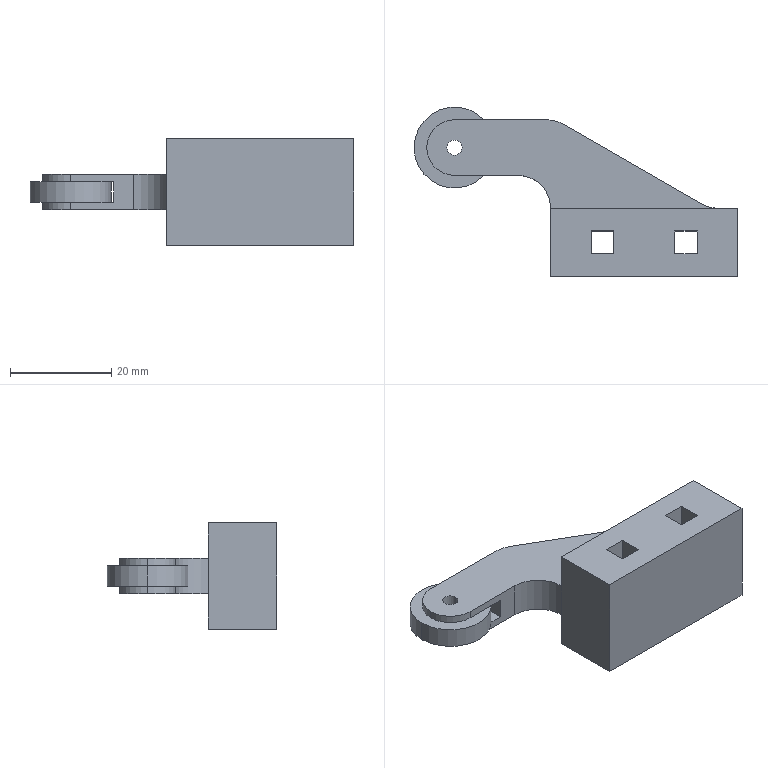Part | SolidWorks | features BaseBody 1 | 1 solid | 48 faces | box 64 x 33.5 x 21 mm | volume 12733 mm3 | plane 37 | cylinder 11 | commonest cylinder face diameters 11 x4 13 x3 3 x2 16 x2
STEP:
#1=CARTESIAN_POINT('',(-48.,25.5,2.));
#2=VERTEX_POINT('',#1);
#3=CARTESIAN_POINT('',(-50.191,31.,2.));
#4=VERTEX_POINT('',#3);
#5=CARTESIAN_POINT('',(-56.,25.5,2.));
#6=DIRECTION('',(0.,0.,1.));
#7=DIRECTION('',(1.,0.,0.));
#8=AXIS2_PLACEMENT_3D('',#5,#6,#7);
#9=CIRCLE('',#8,8.);
#10=EDGE_CURVE('',#2,#4,#9,.T.);
#11=ORIENTED_EDGE('',*,*,#10,.F.);
#12=CARTESIAN_POINT('',(-48.,25.5,-2.));
#13=VERTEX_POINT('',#12);
#14=CARTESIAN_POINT('',(-48.,25.5,2.));
#15=DIRECTION('',(0.,0.,-1.));
#16=VECTOR('',#15,1000.);
#17=LINE('',#14,#16);
#18=EDGE_CURVE('',#2,#13,#17,.T.);
#19=ORIENTED_EDGE('',*,*,#18,.T.);
#20=CARTESIAN_POINT('',(-50.191,31.,-2.));
#21=VERTEX_POINT('',#20);
#22=CARTESIAN_POINT('',(-56.,25.5,-2.));
#23=DIRECTION('',(0.,0.,1.));
#24=DIRECTION('',(-1.,0.,0.));
#25=AXIS2_PLACEMENT_3D('',#22,#23,#24);
#26=CIRCLE('',#25,8.);
#27=EDGE_CURVE('',#13,#21,#26,.T.);
#28=ORIENTED_EDGE('',*,*,#27,.T.);
#29=CARTESIAN_POINT('',(-64.,25.5,-2.));
#30=VERTEX_POINT('',#29);
#31=CARTESIAN_POINT('',(-56.,25.5,-2.));
#32=DIRECTION('',(0.,0.,1.));
#33=DIRECTION('',(1.,0.,0.));
#34=AXIS2_PLACEMENT_3D('',#31,#32,#33);
#35=CIRCLE('',#34,8.);
#36=EDGE_CURVE('',#21,#30,#35,.T.);
#37=ORIENTED_EDGE('',*,*,#36,.T.);
#38=CARTESIAN_POINT('',(-64.,25.5,2.));
#39=VERTEX_POINT('',#38);
#40=CARTESIAN_POINT('',(-64.,25.5,2.));
#41=DIRECTION('',(0.,0.,-1.));
#42=VECTOR('',#41,1000.);
#43=LINE('',#40,#42);
#44=EDGE_CURVE('',#39,#30,#43,.T.);
#45=ORIENTED_EDGE('',*,*,#44,.F.);
#46=CARTESIAN_POINT('',(-56.,25.5,2.));
#47=DIRECTION('',(0.,0.,1.));
#48=DIRECTION('',(1.,0.,0.));
#49=AXIS2_PLACEMENT_3D('',#46,#47,#48);
#50=CIRCLE('',#49,8.);
#51=EDGE_CURVE('',#4,#39,#50,.T.);
#52=ORIENTED_EDGE('',*,*,#51,.F.);
#53=EDGE_LOOP('',(#11,#19,#28,#37,#45,#52));
#54=FACE_OUTER_BOUND('',#53,.T.);
#55=CARTESIAN_POINT('',(-56.,25.5,2.));
#56=DIRECTION('',(0.,0.,-1.));
#57=DIRECTION('',(-1.,0.,0.));
#58=AXIS2_PLACEMENT_3D('',#55,#56,#57);
#59=CYLINDRICAL_SURFACE('',#58,8.);
#60=ADVANCED_FACE('',(#54),#59,.T.);
#61=CARTESIAN_POINT('',(-57.5,25.5,3.5));
#62=VERTEX_POINT('',#61);
#63=CARTESIAN_POINT('',(-54.5,25.5,3.5));
#64=VERTEX_POINT('',#63);
#65=CARTESIAN_POINT('',(-56.,25.5,3.5));
#66=DIRECTION('',(0.,0.,1.));
#67=DIRECTION('',(1.,0.,0.));
#68=AXIS2_PLACEMENT_3D('',#65,#66,#67);
#69=CIRCLE('',#68,1.5);
#70=EDGE_CURVE('',#62,#64,#69,.T.);
#71=ORIENTED_EDGE('',*,*,#70,.T.);
#72=CARTESIAN_POINT('',(-54.5,25.5,-3.5));
#73=VERTEX_POINT('',#72);
#74=CARTESIAN_POINT('',(-54.5,25.5,3.5));
#75=DIRECTION('',(0.,0.,-1.));
#76=VECTOR('',#75,1000.);
#77=LINE('',#74,#76);
#78=EDGE_CURVE('',#64,#73,#77,.T.);
#79=ORIENTED_EDGE('',*,*,#78,.T.);
#80=CARTESIAN_POINT('',(-57.5,25.5,-3.5));
#81=VERTEX_POINT('',#80);
#82=CARTESIAN_POINT('',(-56.,25.5,-3.5));
#83=DIRECTION('',(0.,0.,1.));
#84=DIRECTION('',(1.,0.,0.));
#85=AXIS2_PLACEMENT_3D('',#82,#83,#84);
#86=CIRCLE('',#85,1.5);
#87=EDGE_CURVE('',#81,#73,#86,.T.);
#88=ORIENTED_EDGE('',*,*,#87,.F.);
#89=CARTESIAN_POINT('',(-57.5,25.5,3.5));
#90=DIRECTION('',(0.,0.,-1.));
#91=VECTOR('',#90,1000.);
#92=LINE('',#89,#91);
#93=EDGE_CURVE('',#62,#81,#92,.T.);
#94=ORIENTED_EDGE('',*,*,#93,.F.);
#95=EDGE_LOOP('',(#71,#79,#88,#94));
#96=FACE_OUTER_BOUND('',#95,.T.);
#97=CARTESIAN_POINT('',(-56.,25.5,3.5));
#98=DIRECTION('',(0.,0.,-1.));
#99=DIRECTION('',(-1.,0.,0.));
#100=AXIS2_PLACEMENT_3D('',#97,#98,#99);
#101=CYLINDRICAL_SURFACE('',#100,1.5);
#102=ADVANCED_FACE('',(#96),#101,.F.);
#103=CARTESIAN_POINT('',(-56.,20.,-2.));
#104=VERTEX_POINT('',#103);
#105=CARTESIAN_POINT('',(-61.5,25.5,-2.));
#106=VERTEX_POINT('',#105);
#107=CARTESIAN_POINT('',(-56.,25.5,-2.));
#108=DIRECTION('',(0.,0.,-1.));
#109=DIRECTION('',(-1.,0.,0.));
#110=AXIS2_PLACEMENT_3D('',#107,#108,#109);
#111=CIRCLE('',#110,5.5);
#112=EDGE_CURVE('',#104,#106,#111,.T.);
#113=ORIENTED_EDGE('',*,*,#112,.T.);
#114=CARTESIAN_POINT('',(-61.5,25.5,-3.5));
#115=VERTEX_POINT('',#114);
#116=CARTESIAN_POINT('',(-61.5,25.5,3.5));
#117=DIRECTION('',(0.,0.,-1.));
#118=VECTOR('',#117,1000.);
#119=LINE('',#116,#118);
#120=EDGE_CURVE('',#106,#115,#119,.T.);
#121=ORIENTED_EDGE('',*,*,#120,.T.);
#122=CARTESIAN_POINT('',(-56.,20.,-3.5));
#123=VERTEX_POINT('',#122);
#124=CARTESIAN_POINT('',(-56.,25.5,-3.5));
#125=DIRECTION('',(0.,0.,1.));
#126=DIRECTION('',(1.,0.,0.));
#127=AXIS2_PLACEMENT_3D('',#124,#125,#126);
#128=CIRCLE('',#127,5.5);
#129=EDGE_CURVE('',#115,#123,#128,.T.);
#130=ORIENTED_EDGE('',*,*,#129,.T.);
#131=CARTESIAN_POINT('',(-56.,20.,3.5));
#132=DIRECTION('',(0.,0.,-1.));
#133=VECTOR('',#132,1000.);
#134=LINE('',#131,#133);
#135=EDGE_CURVE('',#104,#123,#134,.T.);
#136=ORIENTED_EDGE('',*,*,#135,.F.);
#137=EDGE_LOOP('',(#113,#121,#130,#136));
#138=FACE_OUTER_BOUND('',#137,.T.);
#139=CARTESIAN_POINT('',(-56.,25.5,3.5));
#140=DIRECTION('',(0.,0.,-1.));
#141=DIRECTION('',(-1.,0.,0.));
#142=AXIS2_PLACEMENT_3D('',#139,#140,#141);
#143=CYLINDRICAL_SURFACE('',#142,5.5);
#144=ADVANCED_FACE('',(#138),#143,.T.);
#145=CARTESIAN_POINT('',(-61.5,25.5,3.5));
#146=VERTEX_POINT('',#145);
#147=CARTESIAN_POINT('',(-56.,20.,3.5));
#148=VERTEX_POINT('',#147);
#149=CARTESIAN_POINT('',(-56.,25.5,3.5));
#150=DIRECTION('',(0.,0.,1.));
#151=DIRECTION('',(1.,0.,0.));
#152=AXIS2_PLACEMENT_3D('',#149,#150,#151);
#153=CIRCLE('',#152,5.5);
#154=EDGE_CURVE('',#146,#148,#153,.T.);
#155=ORIENTED_EDGE('',*,*,#154,.F.);
#156=CARTESIAN_POINT('',(-61.5,25.5,2.));
#157=VERTEX_POINT('',#156);
#158=CARTESIAN_POINT('',(-61.5,25.5,3.5));
#159=DIRECTION('',(0.,0.,-1.));
#160=VECTOR('',#159,1000.);
#161=LINE('',#158,#160);
#162=EDGE_CURVE('',#146,#157,#161,.T.);
#163=ORIENTED_EDGE('',*,*,#162,.T.);
#164=CARTESIAN_POINT('',(-56.,20.,2.));
#165=VERTEX_POINT('',#164);
#166=CARTESIAN_POINT('',(-56.,25.5,2.));
#167=DIRECTION('',(0.,0.,1.));
#168=DIRECTION('',(1.,0.,0.));
#169=AXIS2_PLACEMENT_3D('',#166,#167,#168);
#170=CIRCLE('',#169,5.5);
#171=EDGE_CURVE('',#157,#165,#170,.T.);
#172=ORIENTED_EDGE('',*,*,#171,.T.);
#173=CARTESIAN_POINT('',(-56.,20.,3.5));
#174=DIRECTION('',(0.,0.,-1.));
#175=VECTOR('',#174,1000.);
#176=LINE('',#173,#175);
#177=EDGE_CURVE('',#148,#165,#176,.T.);
#178=ORIENTED_EDGE('',*,*,#177,.F.);
#179=EDGE_LOOP('',(#155,#163,#172,#178));
#180=FACE_OUTER_BOUND('',#179,.T.);
#181=CARTESIAN_POINT('',(-56.,25.5,3.5));
#182=DIRECTION('',(0.,0.,-1.));
#183=DIRECTION('',(-1.,0.,0.));
#184=AXIS2_PLACEMENT_3D('',#181,#182,#183);
#185=CYLINDRICAL_SURFACE('',#184,5.5);
#186=ADVANCED_FACE('',(#180),#185,.T.);
#187=CARTESIAN_POINT('',(-8.,9.,-1.5));
#188=VERTEX_POINT('',#187);
#189=CARTESIAN_POINT('',(-8.,4.5,-1.5));
#190=VERTEX_POINT('',#189);
#191=CARTESIAN_POINT('',(-8.,4.5,-1.5));
#192=DIRECTION('',(0.,-1.,0.));
#193=VECTOR('',#192,1000.);
#194=LINE('',#191,#193);
#195=EDGE_CURVE('',#188,#190,#194,.T.);
#196=ORIENTED_EDGE('',*,*,#195,.F.);
#197=CARTESIAN_POINT('',(-8.,9.,-10.5));
#198=VERTEX_POINT('',#197);
#199=CARTESIAN_POINT('',(-8.,9.,3.5));
#200=DIRECTION('',(0.,0.,-1.));
#201=VECTOR('',#200,1000.);
#202=LINE('',#199,#201);
#203=EDGE_CURVE('',#188,#198,#202,.T.);
#204=ORIENTED_EDGE('',*,*,#203,.T.);
#205=CARTESIAN_POINT('',(-8.,4.5,-10.5));
#206=VERTEX_POINT('',#205);
#207=CARTESIAN_POINT('',(-8.,9.,-10.5));
#208=DIRECTION('',(0.,1.,0.));
#209=VECTOR('',#208,1000.);
#210=LINE('',#207,#209);
#211=EDGE_CURVE('',#206,#198,#210,.T.);
#212=ORIENTED_EDGE('',*,*,#211,.F.);
#213=CARTESIAN_POINT('',(-8.,4.5,3.5));
#214=DIRECTION('',(0.,0.,-1.));
#215=VECTOR('',#214,1000.);
#216=LINE('',#213,#215);
#217=EDGE_CURVE('',#190,#206,#216,.T.);
#218=ORIENTED_EDGE('',*,*,#217,.F.);
#219=EDGE_LOOP('',(#196,#204,#212,#218));
#220=FACE_OUTER_BOUND('',#219,.T.);
#221=CARTESIAN_POINT('',(-8.,4.5,3.5));
#222=DIRECTION('',(-1.,0.,0.));
#223=DIRECTION('',(0.,0.,1.));
#224=AXIS2_PLACEMENT_3D('',#221,#222,#223);
#225=PLANE('',#224);
#226=ADVANCED_FACE('',(#220),#225,.T.);
#227=CARTESIAN_POINT('',(-12.5,9.,-1.5));
#228=VERTEX_POINT('',#227);
#229=CARTESIAN_POINT('',(-12.5,9.,-1.5));
#230=DIRECTION('',(1.,0.,0.));
#231=VECTOR('',#230,1000.);
#232=LINE('',#229,#231);
#233=EDGE_CURVE('',#228,#188,#232,.T.);
#234=ORIENTED_EDGE('',*,*,#233,.F.);
#235=CARTESIAN_POINT('',(-12.5,9.,-10.5));
#236=VERTEX_POINT('',#235);
#237=CARTESIAN_POINT('',(-12.5,9.,3.5));
#238=DIRECTION('',(0.,0.,-1.));
#239=VECTOR('',#238,1000.);
#240=LINE('',#237,#239);
#241=EDGE_CURVE('',#228,#236,#240,.T.);
#242=ORIENTED_EDGE('',*,*,#241,.T.);
#243=CARTESIAN_POINT('',(-12.5,9.,-10.5));
#244=DIRECTION('',(-1.,0.,0.));
#245=VECTOR('',#244,1000.);
#246=LINE('',#243,#245);
#247=EDGE_CURVE('',#198,#236,#246,.T.);
#248=ORIENTED_EDGE('',*,*,#247,.F.);
#249=ORIENTED_EDGE('',*,*,#203,.F.);
#250=EDGE_LOOP('',(#234,#242,#248,#249));
#251=FACE_OUTER_BOUND('',#250,.T.);
#252=CARTESIAN_POINT('',(-12.5,9.,3.5));
#253=DIRECTION('',(0.,-1.,0.));
#254=DIRECTION('',(0.,0.,-1.));
#255=AXIS2_PLACEMENT_3D('',#252,#253,#254);
#256=PLANE('',#255);
#257=ADVANCED_FACE('',(#251),#256,.T.);
#258=CARTESIAN_POINT('',(-12.5,4.5,-1.5));
#259=VERTEX_POINT('',#258);
#260=CARTESIAN_POINT('',(-12.5,4.5,-1.5));
#261=DIRECTION('',(0.,1.,0.));
#262=VECTOR('',#261,1000.);
#263=LINE('',#260,#262);
#264=EDGE_CURVE('',#259,#228,#263,.T.);
#265=ORIENTED_EDGE('',*,*,#264,.F.);
#266=CARTESIAN_POINT('',(-12.5,4.5,-10.5));
#267=VERTEX_POINT('',#266);
#268=CARTESIAN_POINT('',(-12.5,4.5,3.5));
#269=DIRECTION('',(0.,0.,-1.));
#270=VECTOR('',#269,1000.);
#271=LINE('',#268,#270);
#272=EDGE_CURVE('',#259,#267,#271,.T.);
#273=ORIENTED_EDGE('',*,*,#272,.T.);
#274=CARTESIAN_POINT('',(-12.5,9.,-10.5));
#275=DIRECTION('',(0.,-1.,0.));
#276=VECTOR('',#275,1000.);
#277=LINE('',#274,#276);
#278=EDGE_CURVE('',#236,#267,#277,.T.);
#279=ORIENTED_EDGE('',*,*,#278,.F.);
#280=ORIENTED_EDGE('',*,*,#241,.F.);
#281=EDGE_LOOP('',(#265,#273,#279,#280));
#282=FACE_OUTER_BOUND('',#281,.T.);
#283=CARTESIAN_POINT('',(-12.5,4.5,3.5));
#284=DIRECTION('',(1.,0.,0.));
#285=DIRECTION('',(0.,1.,0.));
#286=AXIS2_PLACEMENT_3D('',#283,#284,#285);
#287=PLANE('',#286);
#288=ADVANCED_FACE('',(#282),#287,.T.);
#289=CARTESIAN_POINT('',(-12.5,4.5,-1.5));
#290=DIRECTION('',(-1.,0.,0.));
#291=VECTOR('',#290,1000.);
#292=LINE('',#289,#291);
#293=EDGE_CURVE('',#190,#259,#292,.T.);
#294=ORIENTED_EDGE('',*,*,#293,.F.);
#295=ORIENTED_EDGE('',*,*,#217,.T.);
#296=CARTESIAN_POINT('',(-12.5,4.5,-10.5));
#297=DIRECTION('',(1.,0.,0.));
#298=VECTOR('',#297,1000.);
#299=LINE('',#296,#298);
#300=EDGE_CURVE('',#267,#206,#299,.T.);
#301=ORIENTED_EDGE('',*,*,#300,.F.);
#302=ORIENTED_EDGE('',*,*,#272,.F.);
#303=EDGE_LOOP('',(#294,#295,#301,#302));
#304=FACE_OUTER_BOUND('',#303,.T.);
#305=CARTESIAN_POINT('',(-12.5,4.5,3.5));
#306=DIRECTION('',(0.,1.,0.));
#307=DIRECTION('',(1.,0.,0.));
#308=AXIS2_PLACEMENT_3D('',#305,#306,#307);
#309=PLANE('',#308);
#310=ADVANCED_FACE('',(#304),#309,.T.);
#311=CARTESIAN_POINT('',(-24.5,9.,-1.5));
#312=VERTEX_POINT('',#311);
#313=CARTESIAN_POINT('',(-24.5,4.5,-1.5));
#314=VERTEX_POINT('',#313);
#315=CARTESIAN_POINT('',(-24.5,4.5,-1.5));
#316=DIRECTION('',(0.,-1.,0.));
#317=VECTOR('',#316,1000.);
#318=LINE('',#315,#317);
#319=EDGE_CURVE('',#312,#314,#318,.T.);
#320=ORIENTED_EDGE('',*,*,#319,.F.);
#321=CARTESIAN_POINT('',(-24.5,9.,-10.5));
#322=VERTEX_POINT('',#321);
#323=CARTESIAN_POINT('',(-24.5,9.,3.5));
#324=DIRECTION('',(0.,0.,-1.));
#325=VECTOR('',#324,1000.);
#326=LINE('',#323,#325);
#327=EDGE_CURVE('',#312,#322,#326,.T.);
#328=ORIENTED_EDGE('',*,*,#327,.T.);
#329=CARTESIAN_POINT('',(-24.5,4.5,-10.5));
#330=VERTEX_POINT('',#329);
#331=CARTESIAN_POINT('',(-24.5,9.,-10.5));
#332=DIRECTION('',(0.,1.,0.));
#333=VECTOR('',#332,1000.);
#334=LINE('',#331,#333);
#335=EDGE_CURVE('',#330,#322,#334,.T.);
#336=ORIENTED_EDGE('',*,*,#335,.F.);
#337=CARTESIAN_POINT('',(-24.5,4.5,3.5));
#338=DIRECTION('',(0.,0.,-1.));
#339=VECTOR('',#338,1000.);
#340=LINE('',#337,#339);
#341=EDGE_CURVE('',#314,#330,#340,.T.);
#342=ORIENTED_EDGE('',*,*,#341,.F.);
#343=EDGE_LOOP('',(#320,#328,#336,#342));
#344=FACE_OUTER_BOUND('',#343,.T.);
#345=CARTESIAN_POINT('',(-24.5,4.5,3.5));
#346=DIRECTION('',(-1.,0.,0.));
#347=DIRECTION('',(0.,1.,0.));
#348=AXIS2_PLACEMENT_3D('',#345,#346,#347);
#349=PLANE('',#348);
#350=ADVANCED_FACE('',(#344),#349,.T.);
#351=CARTESIAN_POINT('',(-29.,9.,-1.5));
#352=VERTEX_POINT('',#351);
#353=CARTESIAN_POINT('',(-29.,9.,-1.5));
#354=DIRECTION('',(1.,0.,0.));
#355=VECTOR('',#354,1000.);
#356=LINE('',#353,#355);
#357=EDGE_CURVE('',#352,#312,#356,.T.);
#358=ORIENTED_EDGE('',*,*,#357,.F.);
#359=CARTESIAN_POINT('',(-29.,9.,-10.5));
#360=VERTEX_POINT('',#359);
#361=CARTESIAN_POINT('',(-29.,9.,3.5));
#362=DIRECTION('',(0.,0.,-1.));
#363=VECTOR('',#362,1000.);
#364=LINE('',#361,#363);
#365=EDGE_CURVE('',#352,#360,#364,.T.);
#366=ORIENTED_EDGE('',*,*,#365,.T.);
#367=CARTESIAN_POINT('',(-29.,9.,-10.5));
#368=DIRECTION('',(-1.,0.,0.));
#369=VECTOR('',#368,1000.);
#370=LINE('',#367,#369);
#371=EDGE_CURVE('',#322,#360,#370,.T.);
#372=ORIENTED_EDGE('',*,*,#371,.F.);
#373=ORIENTED_EDGE('',*,*,#327,.F.);
#374=EDGE_LOOP('',(#358,#366,#372,#373));
#375=FACE_OUTER_BOUND('',#374,.T.);
#376=CARTESIAN_POINT('',(-29.,9.,3.5));
#377=DIRECTION('',(0.,-1.,0.));
#378=DIRECTION('',(0.,0.,-1.));
#379=AXIS2_PLACEMENT_3D('',#376,#377,#378);
#380=PLANE('',#379);
#381=ADVANCED_FACE('',(#375),#380,.T.);
#382=CARTESIAN_POINT('',(-29.,4.5,-1.5));
#383=VERTEX_POINT('',#382);
#384=CARTESIAN_POINT('',(-29.,4.5,-1.5));
#385=DIRECTION('',(0.,1.,0.));
#386=VECTOR('',#385,1000.);
#387=LINE('',#384,#386);
#388=EDGE_CURVE('',#383,#352,#387,.T.);
#389=ORIENTED_EDGE('',*,*,#388,.F.);
#390=CARTESIAN_POINT('',(-29.,4.5,-10.5));
#391=VERTEX_POINT('',#390);
#392=CARTESIAN_POINT('',(-29.,4.5,3.5));
#393=DIRECTION('',(0.,0.,-1.));
#394=VECTOR('',#393,1000.);
#395=LINE('',#392,#394);
#396=EDGE_CURVE('',#383,#391,#395,.T.);
#397=ORIENTED_EDGE('',*,*,#396,.T.);
#398=CARTESIAN_POINT('',(-29.,9.,-10.5));
#399=DIRECTION('',(0.,-1.,0.));
#400=VECTOR('',#399,1000.);
#401=LINE('',#398,#400);
#402=EDGE_CURVE('',#360,#391,#401,.T.);
#403=ORIENTED_EDGE('',*,*,#402,.F.);
#404=ORIENTED_EDGE('',*,*,#365,.F.);
#405=EDGE_LOOP('',(#389,#397,#403,#404));
#406=FACE_OUTER_BOUND('',#405,.T.);
#407=CARTESIAN_POINT('',(-29.,4.5,3.5));
#408=DIRECTION('',(1.,0.,0.));
#409=DIRECTION('',(0.,1.,0.));
#410=AXIS2_PLACEMENT_3D('',#407,#408,#409);
#411=PLANE('',#410);
#412=ADVANCED_FACE('',(#406),#411,.T.);
#413=CARTESIAN_POINT('',(-29.,4.5,-1.5));
#414=DIRECTION('',(-1.,0.,0.));
#415=VECTOR('',#414,1000.);
#416=LINE('',#413,#415);
#417=EDGE_CURVE('',#314,#383,#416,.T.);
#418=ORIENTED_EDGE('',*,*,#417,.F.);
#419=ORIENTED_EDGE('',*,*,#341,.T.);
#420=CARTESIAN_POINT('',(-29.,4.5,-10.5));
#421=DIRECTION('',(1.,0.,0.));
#422=VECTOR('',#421,1000.);
#423=LINE('',#420,#422);
#424=EDGE_CURVE('',#391,#330,#423,.T.);
#425=ORIENTED_EDGE('',*,*,#424,.F.);
#426=ORIENTED_EDGE('',*,*,#396,.F.);
#427=EDGE_LOOP('',(#418,#419,#425,#426));
#428=FACE_OUTER_BOUND('',#427,.T.);
#429=CARTESIAN_POINT('',(-29.,4.5,3.5));
#430=DIRECTION('',(0.,1.,0.));
#431=DIRECTION('',(1.,0.,0.));
#432=AXIS2_PLACEMENT_3D('',#429,#430,#431);
#433=PLANE('',#432);
#434=ADVANCED_FACE('',(#428),#433,.T.);
#435=CARTESIAN_POINT('',(-50.191,20.,2.));
#436=VERTEX_POINT('',#435);
#437=CARTESIAN_POINT('',(-56.,25.5,2.));
#438=DIRECTION('',(0.,0.,1.));
#439=DIRECTION('',(1.,0.,0.));
#440=AXIS2_PLACEMENT_3D('',#437,#438,#439);
#441=CIRCLE('',#440,8.);
#442=EDGE_CURVE('',#436,#2,#441,.T.);
#443=ORIENTED_EDGE('',*,*,#442,.T.);
#444=ORIENTED_EDGE('',*,*,#10,.T.);
#445=CARTESIAN_POINT('',(-47.5,31.,2.));
#446=VERTEX_POINT('',#445);
#447=CARTESIAN_POINT('',(-56.,31.,2.));
#448=DIRECTION('',(-1.,0.,0.));
#449=VECTOR('',#448,1000.);
#450=LINE('',#447,#449);
#451=EDGE_CURVE('',#446,#4,#450,.T.);
#452=ORIENTED_EDGE('',*,*,#451,.F.);
#453=CARTESIAN_POINT('',(-47.5,20.,2.));
#454=VERTEX_POINT('',#453);
#455=CARTESIAN_POINT('',(-47.5,0.,2.));
#456=DIRECTION('',(0.,1.,0.));
#457=VECTOR('',#456,1000.);
#458=LINE('',#455,#457);
#459=EDGE_CURVE('',#454,#446,#458,.T.);
#460=ORIENTED_EDGE('',*,*,#459,.F.);
#461=CARTESIAN_POINT('',(-43.5,20.,2.));
#462=DIRECTION('',(1.,0.,0.));
#463=VECTOR('',#462,1000.);
#464=LINE('',#461,#463);
#465=EDGE_CURVE('',#436,#454,#464,.T.);
#466=ORIENTED_EDGE('',*,*,#465,.F.);
#467=EDGE_LOOP('',(#443,#444,#452,#460,#466));
#468=FACE_OUTER_BOUND('',#467,.T.);
#469=CARTESIAN_POINT('',(-67.5,0.,2.));
#470=DIRECTION('',(0.,0.,1.));
#471=DIRECTION('',(1.,0.,0.));
#472=AXIS2_PLACEMENT_3D('',#469,#470,#471);
#473=PLANE('',#472);
#474=ADVANCED_FACE('',(#468),#473,.F.);
#475=CARTESIAN_POINT('',(-50.191,20.,-2.));
#476=VERTEX_POINT('',#475);
#477=CARTESIAN_POINT('',(-56.,25.5,-2.));
#478=DIRECTION('',(0.,0.,1.));
#479=DIRECTION('',(-1.,0.,0.));
#480=AXIS2_PLACEMENT_3D('',#477,#478,#479);
#481=CIRCLE('',#480,8.);
#482=EDGE_CURVE('',#476,#13,#481,.T.);
#483=ORIENTED_EDGE('',*,*,#482,.F.);
#484=CARTESIAN_POINT('',(-47.5,20.,-2.));
#485=VERTEX_POINT('',#484);
#486=CARTESIAN_POINT('',(-43.5,20.,-2.));
#487=DIRECTION('',(-1.,0.,0.));
#488=VECTOR('',#487,1000.);
#489=LINE('',#486,#488);
#490=EDGE_CURVE('',#485,#476,#489,.T.);
#491=ORIENTED_EDGE('',*,*,#490,.F.);
#492=CARTESIAN_POINT('',(-47.5,31.,-2.));
#493=VERTEX_POINT('',#492);
#494=CARTESIAN_POINT('',(-47.5,0.,-2.));
#495=DIRECTION('',(0.,1.,0.));
#496=VECTOR('',#495,1000.);
#497=LINE('',#494,#496);
#498=EDGE_CURVE('',#485,#493,#497,.T.);
#499=ORIENTED_EDGE('',*,*,#498,.T.);
#500=CARTESIAN_POINT('',(-56.,31.,-2.));
#501=DIRECTION('',(1.,0.,0.));
#502=VECTOR('',#501,1000.);
#503=LINE('',#500,#502);
#504=EDGE_CURVE('',#21,#493,#503,.T.);
#505=ORIENTED_EDGE('',*,*,#504,.F.);
#506=ORIENTED_EDGE('',*,*,#27,.F.);
#507=EDGE_LOOP('',(#483,#491,#499,#505,#506));
#508=FACE_OUTER_BOUND('',#507,.T.);
#509=CARTESIAN_POINT('',(-67.5,0.,-2.));
#510=DIRECTION('',(0.,0.,-1.));
#511=DIRECTION('',(0.,-1.,0.));
#512=AXIS2_PLACEMENT_3D('',#509,#510,#511);
#513=PLANE('',#512);
#514=ADVANCED_FACE('',(#508),#513,.F.);
#515=ORIENTED_EDGE('',*,*,#162,.F.);
#516=CARTESIAN_POINT('',(-56.,31.,3.5));
#517=VERTEX_POINT('',#516);
#518=CARTESIAN_POINT('',(-56.,25.5,3.5));
#519=DIRECTION('',(0.,0.,1.));
#520=DIRECTION('',(1.,0.,0.));
#521=AXIS2_PLACEMENT_3D('',#518,#519,#520);
#522=CIRCLE('',#521,5.5);
#523=EDGE_CURVE('',#517,#146,#522,.T.);
#524=ORIENTED_EDGE('',*,*,#523,.F.);
#525=CARTESIAN_POINT('',(-56.,31.,2.));
#526=VERTEX_POINT('',#525);
#527=CARTESIAN_POINT('',(-56.,31.,3.5));
#528=DIRECTION('',(0.,0.,-1.));
#529=VECTOR('',#528,1000.);
#530=LINE('',#527,#529);
#531=EDGE_CURVE('',#517,#526,#530,.T.);
#532=ORIENTED_EDGE('',*,*,#531,.T.);
#533=CARTESIAN_POINT('',(-56.,25.5,2.));
#534=DIRECTION('',(0.,0.,1.));
#535=DIRECTION('',(1.,0.,0.));
#536=AXIS2_PLACEMENT_3D('',#533,#534,#535);
#537=CIRCLE('',#536,5.5);
#538=EDGE_CURVE('',#526,#157,#537,.T.);
#539=ORIENTED_EDGE('',*,*,#538,.T.);
#540=EDGE_LOOP('',(#515,#524,#532,#539));
#541=FACE_OUTER_BOUND('',#540,.T.);
#542=CARTESIAN_POINT('',(-56.,25.5,3.5));
#543=DIRECTION('',(0.,0.,-1.));
#544=DIRECTION('',(-1.,0.,0.));
#545=AXIS2_PLACEMENT_3D('',#542,#543,#544);
#546=CYLINDRICAL_SURFACE('',#545,5.5);
#547=ADVANCED_FACE('',(#541),#546,.T.);
#548=ORIENTED_EDGE('',*,*,#70,.F.);
#549=CARTESIAN_POINT('',(-56.,25.5,3.5));
#550=DIRECTION('',(0.,0.,1.));
#551=DIRECTION('',(1.,0.,0.));
#552=AXIS2_PLACEMENT_3D('',#549,#550,#551);
#553=CIRCLE('',#552,1.5);
#554=EDGE_CURVE('',#64,#62,#553,.T.);
#555=ORIENTED_EDGE('',*,*,#554,.F.);
#556=EDGE_LOOP('',(#548,#555));
#557=FACE_BOUND('',#556,.T.);
#558=CARTESIAN_POINT('',(-4.,13.5,3.5));
#559=VERTEX_POINT('',#558);
#560=CARTESIAN_POINT('',(-37.,13.5,3.5));
#561=VERTEX_POINT('',#560);
#562=CARTESIAN_POINT('',(0.,13.5,3.5));
#563=DIRECTION('',(-1.,0.,0.));
#564=VECTOR('',#563,1000.);
#565=LINE('',#562,#564);
#566=EDGE_CURVE('',#559,#561,#565,.T.);
#567=ORIENTED_EDGE('',*,*,#566,.F.);
#568=CARTESIAN_POINT('',(-7.25,14.371,3.5));
#569=VERTEX_POINT('',#568);
#570=CARTESIAN_POINT('',(-4.,20.,3.5));
#571=DIRECTION('',(0.,0.,-1.));
#572=DIRECTION('',(-1.,0.,0.));
#573=AXIS2_PLACEMENT_3D('',#570,#571,#572);
#574=CIRCLE('',#573,6.5);
#575=EDGE_CURVE('',#559,#569,#574,.T.);
#576=ORIENTED_EDGE('',*,*,#575,.T.);
#577=CARTESIAN_POINT('',(-34.544,30.129,3.5));
#578=VERTEX_POINT('',#577);
#579=CARTESIAN_POINT('',(-34.544,30.129,3.5));
#580=DIRECTION('',(-0.866,0.5,0.));
#581=VECTOR('',#580,1000.);
#582=LINE('',#579,#581);
#583=EDGE_CURVE('',#569,#578,#582,.T.);
#584=ORIENTED_EDGE('',*,*,#583,.T.);
#585=CARTESIAN_POINT('',(-37.794,31.,3.5));
#586=VERTEX_POINT('',#585);
#587=CARTESIAN_POINT('',(-37.794,24.5,3.5));
#588=DIRECTION('',(0.,0.,1.));
#589=DIRECTION('',(1.,0.,0.));
#590=AXIS2_PLACEMENT_3D('',#587,#588,#589);
#591=CIRCLE('',#590,6.5);
#592=EDGE_CURVE('',#578,#586,#591,.T.);
#593=ORIENTED_EDGE('',*,*,#592,.T.);
#594=CARTESIAN_POINT('',(-56.,31.,3.5));
#595=DIRECTION('',(-1.,0.,0.));
#596=VECTOR('',#595,1000.);
#597=LINE('',#594,#596);
#598=EDGE_CURVE('',#586,#517,#597,.T.);
#599=ORIENTED_EDGE('',*,*,#598,.T.);
#600=ORIENTED_EDGE('',*,*,#523,.T.);
#601=ORIENTED_EDGE('',*,*,#154,.T.);
#602=CARTESIAN_POINT('',(-43.5,20.,3.5));
#603=VERTEX_POINT('',#602);
#604=CARTESIAN_POINT('',(-43.5,20.,3.5));
#605=DIRECTION('',(1.,0.,0.));
#606=VECTOR('',#605,1000.);
#607=LINE('',#604,#606);
#608=EDGE_CURVE('',#148,#603,#607,.T.);
#609=ORIENTED_EDGE('',*,*,#608,.T.);
#610=CARTESIAN_POINT('',(-43.5,13.5,3.5));
#611=DIRECTION('',(0.,0.,-1.));
#612=DIRECTION('',(1.,0.,0.));
#613=AXIS2_PLACEMENT_3D('',#610,#611,#612);
#614=CIRCLE('',#613,6.5);
#615=EDGE_CURVE('',#603,#561,#614,.T.);
#616=ORIENTED_EDGE('',*,*,#615,.T.);
#617=EDGE_LOOP('',(#567,#576,#584,#593,#599,#600,#601,#609,#616));
#618=FACE_OUTER_BOUND('',#617,.T.);
#619=CARTESIAN_POINT('',(-43.5,13.5,3.5));
#620=DIRECTION('',(0.,0.,1.));
#621=DIRECTION('',(1.,0.,0.));
#622=AXIS2_PLACEMENT_3D('',#619,#620,#621);
#623=PLANE('',#622);
#624=ADVANCED_FACE('',(#557,#618),#623,.T.);
#625=ORIENTED_EDGE('',*,*,#87,.T.);
#626=CARTESIAN_POINT('',(-56.,25.5,-3.5));
#627=DIRECTION('',(0.,0.,1.));
#628=DIRECTION('',(1.,0.,0.));
#629=AXIS2_PLACEMENT_3D('',#626,#627,#628);
#630=CIRCLE('',#629,1.5);
#631=EDGE_CURVE('',#73,#81,#630,.T.);
#632=ORIENTED_EDGE('',*,*,#631,.T.);
#633=EDGE_LOOP('',(#625,#632));
#634=FACE_BOUND('',#633,.T.);
#635=CARTESIAN_POINT('',(-4.,13.5,-3.5));
#636=VERTEX_POINT('',#635);
#637=CARTESIAN_POINT('',(-7.25,14.371,-3.5));
#638=VERTEX_POINT('',#637);
#639=CARTESIAN_POINT('',(-4.,20.,-3.5));
#640=DIRECTION('',(0.,0.,-1.));
#641=DIRECTION('',(-1.,0.,0.));
#642=AXIS2_PLACEMENT_3D('',#639,#640,#641);
#643=CIRCLE('',#642,6.5);
#644=EDGE_CURVE('',#636,#638,#643,.T.);
#645=ORIENTED_EDGE('',*,*,#644,.F.);
#646=CARTESIAN_POINT('',(-37.,13.5,-3.5));
#647=VERTEX_POINT('',#646);
#648=CARTESIAN_POINT('',(0.,13.5,-3.5));
#649=DIRECTION('',(-1.,0.,0.));
#650=VECTOR('',#649,1000.);
#651=LINE('',#648,#650);
#652=EDGE_CURVE('',#636,#647,#651,.T.);
#653=ORIENTED_EDGE('',*,*,#652,.T.);
#654=CARTESIAN_POINT('',(-43.5,20.,-3.5));
#655=VERTEX_POINT('',#654);
#656=CARTESIAN_POINT('',(-43.5,13.5,-3.5));
#657=DIRECTION('',(0.,0.,-1.));
#658=DIRECTION('',(1.,0.,0.));
#659=AXIS2_PLACEMENT_3D('',#656,#657,#658);
#660=CIRCLE('',#659,6.5);
#661=EDGE_CURVE('',#655,#647,#660,.T.);
#662=ORIENTED_EDGE('',*,*,#661,.F.);
#663=CARTESIAN_POINT('',(-43.5,20.,-3.5));
#664=DIRECTION('',(1.,0.,0.));
#665=VECTOR('',#664,1000.);
#666=LINE('',#663,#665);
#667=EDGE_CURVE('',#123,#655,#666,.T.);
#668=ORIENTED_EDGE('',*,*,#667,.F.);
#669=ORIENTED_EDGE('',*,*,#129,.F.);
#670=CARTESIAN_POINT('',(-56.,31.,-3.5));
#671=VERTEX_POINT('',#670);
#672=CARTESIAN_POINT('',(-56.,25.5,-3.5));
#673=DIRECTION('',(0.,0.,1.));
#674=DIRECTION('',(1.,0.,0.));
#675=AXIS2_PLACEMENT_3D('',#672,#673,#674);
#676=CIRCLE('',#675,5.5);
#677=EDGE_CURVE('',#671,#115,#676,.T.);
#678=ORIENTED_EDGE('',*,*,#677,.F.);
#679=CARTESIAN_POINT('',(-37.794,31.,-3.5));
#680=VERTEX_POINT('',#679);
#681=CARTESIAN_POINT('',(-56.,31.,-3.5));
#682=DIRECTION('',(-1.,0.,0.));
#683=VECTOR('',#682,1000.);
#684=LINE('',#681,#683);
#685=EDGE_CURVE('',#680,#671,#684,.T.);
#686=ORIENTED_EDGE('',*,*,#685,.F.);
#687=CARTESIAN_POINT('',(-34.544,30.129,-3.5));
#688=VERTEX_POINT('',#687);
#689=CARTESIAN_POINT('',(-37.794,24.5,-3.5));
#690=DIRECTION('',(0.,0.,1.));
#691=DIRECTION('',(1.,0.,0.));
#692=AXIS2_PLACEMENT_3D('',#689,#690,#691);
#693=CIRCLE('',#692,6.5);
#694=EDGE_CURVE('',#688,#680,#693,.T.);
#695=ORIENTED_EDGE('',*,*,#694,.F.);
#696=CARTESIAN_POINT('',(-34.544,30.129,-3.5));
#697=DIRECTION('',(-0.866,0.5,0.));
#698=VECTOR('',#697,1000.);
#699=LINE('',#696,#698);
#700=EDGE_CURVE('',#638,#688,#699,.T.);
#701=ORIENTED_EDGE('',*,*,#700,.F.);
#702=EDGE_LOOP('',(#645,#653,#662,#668,#669,#678,#686,#695,#701));
#703=FACE_OUTER_BOUND('',#702,.T.);
#704=CARTESIAN_POINT('',(-43.5,13.5,-3.5));
#705=DIRECTION('',(0.,0.,1.));
#706=DIRECTION('',(1.,0.,0.));
#707=AXIS2_PLACEMENT_3D('',#704,#705,#706);
#708=PLANE('',#707);
#709=ADVANCED_FACE('',(#634,#703),#708,.F.);
#710=CARTESIAN_POINT('',(0.,11.75,-1.5));
#711=VERTEX_POINT('',#710);
#712=CARTESIAN_POINT('',(0.,11.75,1.5));
#713=VERTEX_POINT('',#712);
#714=CARTESIAN_POINT('',(0.,11.75,1.5));
#715=DIRECTION('',(0.,0.,1.));
#716=VECTOR('',#715,1000.);
#717=LINE('',#714,#716);
#718=EDGE_CURVE('',#711,#713,#717,.T.);
#719=ORIENTED_EDGE('',*,*,#718,.F.);
#720=CARTESIAN_POINT('',(0.,1.75,-1.5));
#721=VERTEX_POINT('',#720);
#722=CARTESIAN_POINT('',(0.,1.75,-1.5));
#723=DIRECTION('',(0.,1.,0.));
#724=VECTOR('',#723,1000.);
#725=LINE('',#722,#724);
#726=EDGE_CURVE('',#721,#711,#725,.T.);
#727=ORIENTED_EDGE('',*,*,#726,.F.);
#728=CARTESIAN_POINT('',(0.,1.75,1.5));
#729=VERTEX_POINT('',#728);
#730=CARTESIAN_POINT('',(0.,1.75,1.5));
#731=DIRECTION('',(0.,0.,-1.));
#732=VECTOR('',#731,1000.);
#733=LINE('',#730,#732);
#734=EDGE_CURVE('',#729,#721,#733,.T.);
#735=ORIENTED_EDGE('',*,*,#734,.F.);
#736=CARTESIAN_POINT('',(0.,1.75,1.5));
#737=DIRECTION('',(0.,-1.,0.));
#738=VECTOR('',#737,1000.);
#739=LINE('',#736,#738);
#740=EDGE_CURVE('',#713,#729,#739,.T.);
#741=ORIENTED_EDGE('',*,*,#740,.F.);
#742=EDGE_LOOP('',(#719,#727,#735,#741));
#743=FACE_BOUND('',#742,.T.);
#744=CARTESIAN_POINT('',(0.,0.,10.5));
#745=VERTEX_POINT('',#744);
#746=CARTESIAN_POINT('',(0.,0.,-10.5));
#747=VERTEX_POINT('',#746);
#748=CARTESIAN_POINT('',(0.,0.,3.5));
#749=DIRECTION('',(0.,0.,-1.));
#750=VECTOR('',#749,1000.);
#751=LINE('',#748,#750);
#752=EDGE_CURVE('',#745,#747,#751,.T.);
#753=ORIENTED_EDGE('',*,*,#752,.T.);
#754=CARTESIAN_POINT('',(0.,13.5,-10.5));
#755=VERTEX_POINT('',#754);
#756=CARTESIAN_POINT('',(0.,13.5,-10.5));
#757=DIRECTION('',(0.,1.,0.));
#758=VECTOR('',#757,1000.);
#759=LINE('',#756,#758);
#760=EDGE_CURVE('',#747,#755,#759,.T.);
#761=ORIENTED_EDGE('',*,*,#760,.T.);
#762=CARTESIAN_POINT('',(0.,13.5,10.5));
#763=VERTEX_POINT('',#762);
#764=CARTESIAN_POINT('',(0.,13.5,3.5));
#765=DIRECTION('',(0.,0.,-1.));
#766=VECTOR('',#765,1000.);
#767=LINE('',#764,#766);
#768=EDGE_CURVE('',#763,#755,#767,.T.);
#769=ORIENTED_EDGE('',*,*,#768,.F.);
#770=CARTESIAN_POINT('',(0.,13.5,10.5));
#771=DIRECTION('',(0.,1.,0.));
#772=VECTOR('',#771,1000.);
#773=LINE('',#770,#772);
#774=EDGE_CURVE('',#745,#763,#773,.T.);
#775=ORIENTED_EDGE('',*,*,#774,.F.);
#776=EDGE_LOOP('',(#753,#761,#769,#775));
#777=FACE_OUTER_BOUND('',#776,.T.);
#778=CARTESIAN_POINT('',(0.,13.5,3.5));
#779=DIRECTION('',(-1.,0.,0.));
#780=DIRECTION('',(0.,1.,0.));
#781=AXIS2_PLACEMENT_3D('',#778,#779,#780);
#782=PLANE('',#781);
#783=ADVANCED_FACE('',(#743,#777),#782,.F.);
#784=ORIENTED_EDGE('',*,*,#768,.T.);
#785=CARTESIAN_POINT('',(-37.,13.5,-10.5));
#786=VERTEX_POINT('',#785);
#787=CARTESIAN_POINT('',(0.,13.5,-10.5));
#788=DIRECTION('',(-1.,0.,0.));
#789=VECTOR('',#788,1000.);
#790=LINE('',#787,#789);
#791=EDGE_CURVE('',#755,#786,#790,.T.);
#792=ORIENTED_EDGE('',*,*,#791,.T.);
#793=CARTESIAN_POINT('',(-37.,13.5,-10.5));
#794=DIRECTION('',(0.,0.,1.));
#795=VECTOR('',#794,1000.);
#796=LINE('',#793,#795);
#797=EDGE_CURVE('',#786,#647,#796,.T.);
#798=ORIENTED_EDGE('',*,*,#797,.T.);
#799=ORIENTED_EDGE('',*,*,#652,.F.);
#800=CARTESIAN_POINT('',(-4.,13.5,3.5));
#801=DIRECTION('',(0.,0.,-1.));
#802=VECTOR('',#801,1000.);
#803=LINE('',#800,#802);
#804=EDGE_CURVE('',#559,#636,#803,.T.);
#805=ORIENTED_EDGE('',*,*,#804,.F.);
#806=ORIENTED_EDGE('',*,*,#566,.T.);
#807=CARTESIAN_POINT('',(-37.,13.5,10.5));
#808=VERTEX_POINT('',#807);
#809=CARTESIAN_POINT('',(-37.,13.5,10.5));
#810=DIRECTION('',(0.,0.,-1.));
#811=VECTOR('',#810,1000.);
#812=LINE('',#809,#811);
#813=EDGE_CURVE('',#808,#561,#812,.T.);
#814=ORIENTED_EDGE('',*,*,#813,.F.);
#815=CARTESIAN_POINT('',(0.,13.5,10.5));
#816=DIRECTION('',(-1.,0.,0.));
#817=VECTOR('',#816,1000.);
#818=LINE('',#815,#817);
#819=EDGE_CURVE('',#763,#808,#818,.T.);
#820=ORIENTED_EDGE('',*,*,#819,.F.);
#821=EDGE_LOOP('',(#784,#792,#798,#799,#805,#806,#814,#820));
#822=FACE_OUTER_BOUND('',#821,.T.);
#823=CARTESIAN_POINT('',(-4.,13.5,3.5));
#824=DIRECTION('',(0.,-1.,0.));
#825=DIRECTION('',(0.,0.,-1.));
#826=AXIS2_PLACEMENT_3D('',#823,#824,#825);
#827=PLANE('',#826);
#828=ADVANCED_FACE('',(#822),#827,.F.);
#829=ORIENTED_EDGE('',*,*,#644,.T.);
#830=CARTESIAN_POINT('',(-7.25,14.371,3.5));
#831=DIRECTION('',(0.,0.,-1.));
#832=VECTOR('',#831,1000.);
#833=LINE('',#830,#832);
#834=EDGE_CURVE('',#569,#638,#833,.T.);
#835=ORIENTED_EDGE('',*,*,#834,.F.);
#836=ORIENTED_EDGE('',*,*,#575,.F.);
#837=ORIENTED_EDGE('',*,*,#804,.T.);
#838=EDGE_LOOP('',(#829,#835,#836,#837));
#839=FACE_OUTER_BOUND('',#838,.T.);
#840=CARTESIAN_POINT('',(-4.,20.,3.5));
#841=DIRECTION('',(0.,0.,-1.));
#842=DIRECTION('',(-1.,0.,0.));
#843=AXIS2_PLACEMENT_3D('',#840,#841,#842);
#844=CYLINDRICAL_SURFACE('',#843,6.5);
#845=ADVANCED_FACE('',(#839),#844,.F.);
#846=ORIENTED_EDGE('',*,*,#700,.T.);
#847=CARTESIAN_POINT('',(-34.544,30.129,3.5));
#848=DIRECTION('',(0.,0.,-1.));
#849=VECTOR('',#848,1000.);
#850=LINE('',#847,#849);
#851=EDGE_CURVE('',#578,#688,#850,.T.);
#852=ORIENTED_EDGE('',*,*,#851,.F.);
#853=ORIENTED_EDGE('',*,*,#583,.F.);
#854=ORIENTED_EDGE('',*,*,#834,.T.);
#855=EDGE_LOOP('',(#846,#852,#853,#854));
#856=FACE_OUTER_BOUND('',#855,.T.);
#857=CARTESIAN_POINT('',(-34.544,30.129,3.5));
#858=DIRECTION('',(-0.5,-0.866,0.));
#859=DIRECTION('',(-0.866,0.5,0.));
#860=AXIS2_PLACEMENT_3D('',#857,#858,#859);
#861=PLANE('',#860);
#862=ADVANCED_FACE('',(#856),#861,.F.);
#863=ORIENTED_EDGE('',*,*,#694,.T.);
#864=CARTESIAN_POINT('',(-37.794,31.,3.5));
#865=DIRECTION('',(0.,0.,-1.));
#866=VECTOR('',#865,1000.);
#867=LINE('',#864,#866);
#868=EDGE_CURVE('',#586,#680,#867,.T.);
#869=ORIENTED_EDGE('',*,*,#868,.F.);
#870=ORIENTED_EDGE('',*,*,#592,.F.);
#871=ORIENTED_EDGE('',*,*,#851,.T.);
#872=EDGE_LOOP('',(#863,#869,#870,#871));
#873=FACE_OUTER_BOUND('',#872,.T.);
#874=CARTESIAN_POINT('',(-37.794,24.5,3.5));
#875=DIRECTION('',(0.,0.,-1.));
#876=DIRECTION('',(-1.,0.,0.));
#877=AXIS2_PLACEMENT_3D('',#874,#875,#876);
#878=CYLINDRICAL_SURFACE('',#877,6.5);
#879=ADVANCED_FACE('',(#873),#878,.T.);
#880=CARTESIAN_POINT('',(-47.5,31.,3.5));
#881=DIRECTION('',(0.,0.,1.));
#882=VECTOR('',#881,1000.);
#883=LINE('',#880,#882);
#884=EDGE_CURVE('',#493,#446,#883,.T.);
#885=ORIENTED_EDGE('',*,*,#884,.T.);
#886=ORIENTED_EDGE('',*,*,#451,.T.);
#887=CARTESIAN_POINT('',(-56.,31.,2.));
#888=DIRECTION('',(-1.,0.,0.));
#889=VECTOR('',#888,1000.);
#890=LINE('',#887,#889);
#891=EDGE_CURVE('',#4,#526,#890,.T.);
#892=ORIENTED_EDGE('',*,*,#891,.T.);
#893=ORIENTED_EDGE('',*,*,#531,.F.);
#894=ORIENTED_EDGE('',*,*,#598,.F.);
#895=ORIENTED_EDGE('',*,*,#868,.T.);
#896=ORIENTED_EDGE('',*,*,#685,.T.);
#897=CARTESIAN_POINT('',(-56.,31.,-2.));
#898=VERTEX_POINT('',#897);
#899=CARTESIAN_POINT('',(-56.,31.,3.5));
#900=DIRECTION('',(0.,0.,-1.));
#901=VECTOR('',#900,1000.);
#902=LINE('',#899,#901);
#903=EDGE_CURVE('',#898,#671,#902,.T.);
#904=ORIENTED_EDGE('',*,*,#903,.F.);
#905=CARTESIAN_POINT('',(-56.,31.,-2.));
#906=DIRECTION('',(1.,0.,0.));
#907=VECTOR('',#906,1000.);
#908=LINE('',#905,#907);
#909=EDGE_CURVE('',#898,#21,#908,.T.);
#910=ORIENTED_EDGE('',*,*,#909,.T.);
#911=ORIENTED_EDGE('',*,*,#504,.T.);
#912=EDGE_LOOP('',(#885,#886,#892,#893,#894,#895,#896,#904,#910,#911));
#913=FACE_OUTER_BOUND('',#912,.T.);
#914=CARTESIAN_POINT('',(-56.,31.,3.5));
#915=DIRECTION('',(0.,-1.,0.));
#916=DIRECTION('',(0.,0.,-1.));
#917=AXIS2_PLACEMENT_3D('',#914,#915,#916);
#918=PLANE('',#917);
#919=ADVANCED_FACE('',(#913),#918,.F.);
#920=ORIENTED_EDGE('',*,*,#120,.F.);
#921=CARTESIAN_POINT('',(-56.,25.5,-2.));
#922=DIRECTION('',(0.,0.,-1.));
#923=DIRECTION('',(-1.,0.,0.));
#924=AXIS2_PLACEMENT_3D('',#921,#922,#923);
#925=CIRCLE('',#924,5.5);
#926=EDGE_CURVE('',#106,#898,#925,.T.);
#927=ORIENTED_EDGE('',*,*,#926,.T.);
#928=ORIENTED_EDGE('',*,*,#903,.T.);
#929=ORIENTED_EDGE('',*,*,#677,.T.);
#930=EDGE_LOOP('',(#920,#927,#928,#929));
#931=FACE_OUTER_BOUND('',#930,.T.);
#932=CARTESIAN_POINT('',(-56.,25.5,3.5));
#933=DIRECTION('',(0.,0.,-1.));
#934=DIRECTION('',(-1.,0.,0.));
#935=AXIS2_PLACEMENT_3D('',#932,#933,#934);
#936=CYLINDRICAL_SURFACE('',#935,5.5);
#937=ADVANCED_FACE('',(#931),#936,.T.);
#938=ORIENTED_EDGE('',*,*,#177,.T.);
#939=CARTESIAN_POINT('',(-43.5,20.,2.));
#940=DIRECTION('',(1.,0.,0.));
#941=VECTOR('',#940,1000.);
#942=LINE('',#939,#941);
#943=EDGE_CURVE('',#165,#436,#942,.T.);
#944=ORIENTED_EDGE('',*,*,#943,.T.);
#945=ORIENTED_EDGE('',*,*,#465,.T.);
#946=CARTESIAN_POINT('',(-47.5,20.,3.5));
#947=DIRECTION('',(0.,0.,-1.));
#948=VECTOR('',#947,1000.);
#949=LINE('',#946,#948);
#950=EDGE_CURVE('',#454,#485,#949,.T.);
#951=ORIENTED_EDGE('',*,*,#950,.T.);
#952=ORIENTED_EDGE('',*,*,#490,.T.);
#953=CARTESIAN_POINT('',(-43.5,20.,-2.));
#954=DIRECTION('',(-1.,0.,0.));
#955=VECTOR('',#954,1000.);
#956=LINE('',#953,#955);
#957=EDGE_CURVE('',#476,#104,#956,.T.);
#958=ORIENTED_EDGE('',*,*,#957,.T.);
#959=ORIENTED_EDGE('',*,*,#135,.T.);
#960=ORIENTED_EDGE('',*,*,#667,.T.);
#961=CARTESIAN_POINT('',(-43.5,20.,3.5));
#962=DIRECTION('',(0.,0.,-1.));
#963=VECTOR('',#962,1000.);
#964=LINE('',#961,#963);
#965=EDGE_CURVE('',#603,#655,#964,.T.);
#966=ORIENTED_EDGE('',*,*,#965,.F.);
#967=ORIENTED_EDGE('',*,*,#608,.F.);
#968=EDGE_LOOP('',(#938,#944,#945,#951,#952,#958,#959,#960,#966,#967));
#969=FACE_OUTER_BOUND('',#968,.T.);
#970=CARTESIAN_POINT('',(-43.5,20.,3.5));
#971=DIRECTION('',(0.,1.,0.));
#972=DIRECTION('',(1.,0.,0.));
#973=AXIS2_PLACEMENT_3D('',#970,#971,#972);
#974=PLANE('',#973);
#975=ADVANCED_FACE('',(#969),#974,.F.);
#976=ORIENTED_EDGE('',*,*,#661,.T.);
#977=CARTESIAN_POINT('',(-37.,13.5,3.5));
#978=DIRECTION('',(0.,0.,-1.));
#979=VECTOR('',#978,1000.);
#980=LINE('',#977,#979);
#981=EDGE_CURVE('',#561,#647,#980,.T.);
#982=ORIENTED_EDGE('',*,*,#981,.F.);
#983=ORIENTED_EDGE('',*,*,#615,.F.);
#984=ORIENTED_EDGE('',*,*,#965,.T.);
#985=EDGE_LOOP('',(#976,#982,#983,#984));
#986=FACE_OUTER_BOUND('',#985,.T.);
#987=CARTESIAN_POINT('',(-43.5,13.5,3.5));
#988=DIRECTION('',(0.,0.,-1.));
#989=DIRECTION('',(-1.,0.,0.));
#990=AXIS2_PLACEMENT_3D('',#987,#988,#989);
#991=CYLINDRICAL_SURFACE('',#990,6.5);
#992=ADVANCED_FACE('',(#986),#991,.F.);
#993=ORIENTED_EDGE('',*,*,#981,.T.);
#994=ORIENTED_EDGE('',*,*,#797,.F.);
#995=CARTESIAN_POINT('',(-37.,0.,-10.5));
#996=VERTEX_POINT('',#995);
#997=CARTESIAN_POINT('',(-37.,13.5,-10.5));
#998=DIRECTION('',(0.,-1.,0.));
#999=VECTOR('',#998,1000.);
#1000=LINE('',#997,#999);
#1001=EDGE_CURVE('',#786,#996,#1000,.T.);
#1002=ORIENTED_EDGE('',*,*,#1001,.T.);
#1003=CARTESIAN_POINT('',(-37.,0.,10.5));
#1004=VERTEX_POINT('',#1003);
#1005=CARTESIAN_POINT('',(-37.,0.,3.5));
#1006=DIRECTION('',(0.,0.,-1.));
#1007=VECTOR('',#1006,1000.);
#1008=LINE('',#1005,#1007);
#1009=EDGE_CURVE('',#1004,#996,#1008,.T.);
#1010=ORIENTED_EDGE('',*,*,#1009,.F.);
#1011=CARTESIAN_POINT('',(-37.,13.5,10.5));
#1012=DIRECTION('',(0.,-1.,0.));
#1013=VECTOR('',#1012,1000.);
#1014=LINE('',#1011,#1013);
#1015=EDGE_CURVE('',#808,#1004,#1014,.T.);
#1016=ORIENTED_EDGE('',*,*,#1015,.F.);
#1017=ORIENTED_EDGE('',*,*,#813,.T.);
#1018=EDGE_LOOP('',(#993,#994,#1002,#1010,#1016,#1017));
#1019=FACE_OUTER_BOUND('',#1018,.T.);
#1020=CARTESIAN_POINT('',(-37.,0.,3.5));
#1021=DIRECTION('',(1.,0.,0.));
#1022=DIRECTION('',(0.,1.,0.));
#1023=AXIS2_PLACEMENT_3D('',#1020,#1021,#1022);
#1024=PLANE('',#1023);
#1025=ADVANCED_FACE('',(#1019),#1024,.F.);
#1026=ORIENTED_EDGE('',*,*,#1009,.T.);
#1027=CARTESIAN_POINT('',(0.,0.,-10.5));
#1028=DIRECTION('',(1.,0.,0.));
#1029=VECTOR('',#1028,1000.);
#1030=LINE('',#1027,#1029);
#1031=EDGE_CURVE('',#996,#747,#1030,.T.);
#1032=ORIENTED_EDGE('',*,*,#1031,.T.);
#1033=ORIENTED_EDGE('',*,*,#752,.F.);
#1034=CARTESIAN_POINT('',(0.,0.,10.5));
#1035=DIRECTION('',(1.,0.,0.));
#1036=VECTOR('',#1035,1000.);
#1037=LINE('',#1034,#1036);
#1038=EDGE_CURVE('',#1004,#745,#1037,.T.);
#1039=ORIENTED_EDGE('',*,*,#1038,.F.);
#1040=EDGE_LOOP('',(#1026,#1032,#1033,#1039));
#1041=FACE_OUTER_BOUND('',#1040,.T.);
#1042=CARTESIAN_POINT('',(0.,0.,3.5));
#1043=DIRECTION('',(0.,1.,0.));
#1044=DIRECTION('',(1.,0.,0.));
#1045=AXIS2_PLACEMENT_3D('',#1042,#1043,#1044);
#1046=PLANE('',#1045);
#1047=ADVANCED_FACE('',(#1041),#1046,.F.);
#1048=ORIENTED_EDGE('',*,*,#78,.F.);
#1049=ORIENTED_EDGE('',*,*,#554,.T.);
#1050=ORIENTED_EDGE('',*,*,#93,.T.);
#1051=ORIENTED_EDGE('',*,*,#631,.F.);
#1052=EDGE_LOOP('',(#1048,#1049,#1050,#1051));
#1053=FACE_OUTER_BOUND('',#1052,.T.);
#1054=CARTESIAN_POINT('',(-56.,25.5,3.5));
#1055=DIRECTION('',(0.,0.,-1.));
#1056=DIRECTION('',(-1.,0.,0.));
#1057=AXIS2_PLACEMENT_3D('',#1054,#1055,#1056);
#1058=CYLINDRICAL_SURFACE('',#1057,1.5);
#1059=ADVANCED_FACE('',(#1053),#1058,.F.);
#1060=CARTESIAN_POINT('',(-8.,4.5,1.5));
#1061=VERTEX_POINT('',#1060);
#1062=CARTESIAN_POINT('',(-8.,9.,1.5));
#1063=VERTEX_POINT('',#1062);
#1064=CARTESIAN_POINT('',(-8.,4.5,1.5));
#1065=DIRECTION('',(0.,1.,0.));
#1066=VECTOR('',#1065,1000.);
#1067=LINE('',#1064,#1066);
#1068=EDGE_CURVE('',#1061,#1063,#1067,.T.);
#1069=ORIENTED_EDGE('',*,*,#1068,.F.);
#1070=CARTESIAN_POINT('',(-8.,4.5,10.5));
#1071=VERTEX_POINT('',#1070);
#1072=CARTESIAN_POINT('',(-8.,4.5,3.5));
#1073=DIRECTION('',(0.,0.,-1.));
#1074=VECTOR('',#1073,1000.);
#1075=LINE('',#1072,#1074);
#1076=EDGE_CURVE('',#1071,#1061,#1075,.T.);
#1077=ORIENTED_EDGE('',*,*,#1076,.F.);
#1078=CARTESIAN_POINT('',(-8.,9.,10.5));
#1079=VERTEX_POINT('',#1078);
#1080=CARTESIAN_POINT('',(-8.,9.,10.5));
#1081=DIRECTION('',(0.,1.,0.));
#1082=VECTOR('',#1081,1000.);
#1083=LINE('',#1080,#1082);
#1084=EDGE_CURVE('',#1071,#1079,#1083,.T.);
#1085=ORIENTED_EDGE('',*,*,#1084,.T.);
#1086=CARTESIAN_POINT('',(-8.,9.,3.5));
#1087=DIRECTION('',(0.,0.,-1.));
#1088=VECTOR('',#1087,1000.);
#1089=LINE('',#1086,#1088);
#1090=EDGE_CURVE('',#1079,#1063,#1089,.T.);
#1091=ORIENTED_EDGE('',*,*,#1090,.T.);
#1092=EDGE_LOOP('',(#1069,#1077,#1085,#1091));
#1093=FACE_OUTER_BOUND('',#1092,.T.);
#1094=CARTESIAN_POINT('',(-8.,4.5,3.5));
#1095=DIRECTION('',(-1.,0.,0.));
#1096=DIRECTION('',(0.,0.,1.));
#1097=AXIS2_PLACEMENT_3D('',#1094,#1095,#1096);
#1098=PLANE('',#1097);
#1099=ADVANCED_FACE('',(#1093),#1098,.T.);
#1100=CARTESIAN_POINT('',(-12.5,9.,1.5));
#1101=VERTEX_POINT('',#1100);
#1102=CARTESIAN_POINT('',(-12.5,9.,1.5));
#1103=DIRECTION('',(-1.,0.,0.));
#1104=VECTOR('',#1103,1000.);
#1105=LINE('',#1102,#1104);
#1106=EDGE_CURVE('',#1063,#1101,#1105,.T.);
#1107=ORIENTED_EDGE('',*,*,#1106,.F.);
#1108=ORIENTED_EDGE('',*,*,#1090,.F.);
#1109=CARTESIAN_POINT('',(-12.5,9.,10.5));
#1110=VERTEX_POINT('',#1109);
#1111=CARTESIAN_POINT('',(-12.5,9.,10.5));
#1112=DIRECTION('',(-1.,0.,0.));
#1113=VECTOR('',#1112,1000.);
#1114=LINE('',#1111,#1113);
#1115=EDGE_CURVE('',#1079,#1110,#1114,.T.);
#1116=ORIENTED_EDGE('',*,*,#1115,.T.);
#1117=CARTESIAN_POINT('',(-12.5,9.,3.5));
#1118=DIRECTION('',(0.,0.,-1.));
#1119=VECTOR('',#1118,1000.);
#1120=LINE('',#1117,#1119);
#1121=EDGE_CURVE('',#1110,#1101,#1120,.T.);
#1122=ORIENTED_EDGE('',*,*,#1121,.T.);
#1123=EDGE_LOOP('',(#1107,#1108,#1116,#1122));
#1124=FACE_OUTER_BOUND('',#1123,.T.);
#1125=CARTESIAN_POINT('',(-12.5,9.,3.5));
#1126=DIRECTION('',(0.,-1.,0.));
#1127=DIRECTION('',(0.,0.,-1.));
#1128=AXIS2_PLACEMENT_3D('',#1125,#1126,#1127);
#1129=PLANE('',#1128);
#1130=ADVANCED_FACE('',(#1124),#1129,.T.);
#1131=CARTESIAN_POINT('',(-12.5,4.5,1.5));
#1132=VERTEX_POINT('',#1131);
#1133=CARTESIAN_POINT('',(-12.5,4.5,1.5));
#1134=DIRECTION('',(0.,-1.,0.));
#1135=VECTOR('',#1134,1000.);
#1136=LINE('',#1133,#1135);
#1137=EDGE_CURVE('',#1101,#1132,#1136,.T.);
#1138=ORIENTED_EDGE('',*,*,#1137,.F.);
#1139=ORIENTED_EDGE('',*,*,#1121,.F.);
#1140=CARTESIAN_POINT('',(-12.5,4.5,10.5));
#1141=VERTEX_POINT('',#1140);
#1142=CARTESIAN_POINT('',(-12.5,9.,10.5));
#1143=DIRECTION('',(0.,-1.,0.));
#1144=VECTOR('',#1143,1000.);
#1145=LINE('',#1142,#1144);
#1146=EDGE_CURVE('',#1110,#1141,#1145,.T.);
#1147=ORIENTED_EDGE('',*,*,#1146,.T.);
#1148=CARTESIAN_POINT('',(-12.5,4.5,3.5));
#1149=DIRECTION('',(0.,0.,-1.));
#1150=VECTOR('',#1149,1000.);
#1151=LINE('',#1148,#1150);
#1152=EDGE_CURVE('',#1141,#1132,#1151,.T.);
#1153=ORIENTED_EDGE('',*,*,#1152,.T.);
#1154=EDGE_LOOP('',(#1138,#1139,#1147,#1153));
#1155=FACE_OUTER_BOUND('',#1154,.T.);
#1156=CARTESIAN_POINT('',(-12.5,4.5,3.5));
#1157=DIRECTION('',(1.,0.,0.));
#1158=DIRECTION('',(0.,1.,0.));
#1159=AXIS2_PLACEMENT_3D('',#1156,#1157,#1158);
#1160=PLANE('',#1159);
#1161=ADVANCED_FACE('',(#1155),#1160,.T.);
#1162=CARTESIAN_POINT('',(-12.5,4.5,1.5));
#1163=DIRECTION('',(1.,0.,0.));
#1164=VECTOR('',#1163,1000.);
#1165=LINE('',#1162,#1164);
#1166=EDGE_CURVE('',#1132,#1061,#1165,.T.);
#1167=ORIENTED_EDGE('',*,*,#1166,.F.);
#1168=ORIENTED_EDGE('',*,*,#1152,.F.);
#1169=CARTESIAN_POINT('',(-12.5,4.5,10.5));
#1170=DIRECTION('',(1.,0.,0.));
#1171=VECTOR('',#1170,1000.);
#1172=LINE('',#1169,#1171);
#1173=EDGE_CURVE('',#1141,#1071,#1172,.T.);
#1174=ORIENTED_EDGE('',*,*,#1173,.T.);
#1175=ORIENTED_EDGE('',*,*,#1076,.T.);
#1176=EDGE_LOOP('',(#1167,#1168,#1174,#1175));
#1177=FACE_OUTER_BOUND('',#1176,.T.);
#1178=CARTESIAN_POINT('',(-12.5,4.5,3.5));
#1179=DIRECTION('',(0.,1.,0.));
#1180=DIRECTION('',(1.,0.,0.));
#1181=AXIS2_PLACEMENT_3D('',#1178,#1179,#1180);
#1182=PLANE('',#1181);
#1183=ADVANCED_FACE('',(#1177),#1182,.T.);
#1184=CARTESIAN_POINT('',(-24.5,4.5,1.5));
#1185=VERTEX_POINT('',#1184);
#1186=CARTESIAN_POINT('',(-24.5,9.,1.5));
#1187=VERTEX_POINT('',#1186);
#1188=CARTESIAN_POINT('',(-24.5,4.5,1.5));
#1189=DIRECTION('',(0.,1.,0.));
#1190=VECTOR('',#1189,1000.);
#1191=LINE('',#1188,#1190);
#1192=EDGE_CURVE('',#1185,#1187,#1191,.T.);
#1193=ORIENTED_EDGE('',*,*,#1192,.F.);
#1194=CARTESIAN_POINT('',(-24.5,4.5,10.5));
#1195=VERTEX_POINT('',#1194);
#1196=CARTESIAN_POINT('',(-24.5,4.5,3.5));
#1197=DIRECTION('',(0.,0.,-1.));
#1198=VECTOR('',#1197,1000.);
#1199=LINE('',#1196,#1198);
#1200=EDGE_CURVE('',#1195,#1185,#1199,.T.);
#1201=ORIENTED_EDGE('',*,*,#1200,.F.);
#1202=CARTESIAN_POINT('',(-24.5,9.,10.5));
#1203=VERTEX_POINT('',#1202);
#1204=CARTESIAN_POINT('',(-24.5,9.,10.5));
#1205=DIRECTION('',(0.,1.,0.));
#1206=VECTOR('',#1205,1000.);
#1207=LINE('',#1204,#1206);
#1208=EDGE_CURVE('',#1195,#1203,#1207,.T.);
#1209=ORIENTED_EDGE('',*,*,#1208,.T.);
#1210=CARTESIAN_POINT('',(-24.5,9.,3.5));
#1211=DIRECTION('',(0.,0.,-1.));
#1212=VECTOR('',#1211,1000.);
#1213=LINE('',#1210,#1212);
#1214=EDGE_CURVE('',#1203,#1187,#1213,.T.);
#1215=ORIENTED_EDGE('',*,*,#1214,.T.);
#1216=EDGE_LOOP('',(#1193,#1201,#1209,#1215));
#1217=FACE_OUTER_BOUND('',#1216,.T.);
#1218=CARTESIAN_POINT('',(-24.5,4.5,3.5));
#1219=DIRECTION('',(-1.,0.,0.));
#1220=DIRECTION('',(0.,1.,0.));
#1221=AXIS2_PLACEMENT_3D('',#1218,#1219,#1220);
#1222=PLANE('',#1221);
#1223=ADVANCED_FACE('',(#1217),#1222,.T.);
#1224=CARTESIAN_POINT('',(-29.,9.,1.5));
#1225=VERTEX_POINT('',#1224);
#1226=CARTESIAN_POINT('',(-29.,9.,1.5));
#1227=DIRECTION('',(-1.,0.,0.));
#1228=VECTOR('',#1227,1000.);
#1229=LINE('',#1226,#1228);
#1230=EDGE_CURVE('',#1187,#1225,#1229,.T.);
#1231=ORIENTED_EDGE('',*,*,#1230,.F.);
#1232=ORIENTED_EDGE('',*,*,#1214,.F.);
#1233=CARTESIAN_POINT('',(-29.,9.,10.5));
#1234=VERTEX_POINT('',#1233);
#1235=CARTESIAN_POINT('',(-29.,9.,10.5));
#1236=DIRECTION('',(-1.,0.,0.));
#1237=VECTOR('',#1236,1000.);
#1238=LINE('',#1235,#1237);
#1239=EDGE_CURVE('',#1203,#1234,#1238,.T.);
#1240=ORIENTED_EDGE('',*,*,#1239,.T.);
#1241=CARTESIAN_POINT('',(-29.,9.,3.5));
#1242=DIRECTION('',(0.,0.,-1.));
#1243=VECTOR('',#1242,1000.);
#1244=LINE('',#1241,#1243);
#1245=EDGE_CURVE('',#1234,#1225,#1244,.T.);
#1246=ORIENTED_EDGE('',*,*,#1245,.T.);
#1247=EDGE_LOOP('',(#1231,#1232,#1240,#1246));
#1248=FACE_OUTER_BOUND('',#1247,.T.);
#1249=CARTESIAN_POINT('',(-29.,9.,3.5));
#1250=DIRECTION('',(0.,-1.,0.));
#1251=DIRECTION('',(0.,0.,-1.));
#1252=AXIS2_PLACEMENT_3D('',#1249,#1250,#1251);
#1253=PLANE('',#1252);
#1254=ADVANCED_FACE('',(#1248),#1253,.T.);
#1255=CARTESIAN_POINT('',(-29.,4.5,1.5));
#1256=VERTEX_POINT('',#1255);
#1257=CARTESIAN_POINT('',(-29.,4.5,1.5));
#1258=DIRECTION('',(0.,-1.,0.));
#1259=VECTOR('',#1258,1000.);
#1260=LINE('',#1257,#1259);
#1261=EDGE_CURVE('',#1225,#1256,#1260,.T.);
#1262=ORIENTED_EDGE('',*,*,#1261,.F.);
#1263=ORIENTED_EDGE('',*,*,#1245,.F.);
#1264=CARTESIAN_POINT('',(-29.,4.5,10.5));
#1265=VERTEX_POINT('',#1264);
#1266=CARTESIAN_POINT('',(-29.,9.,10.5));
#1267=DIRECTION('',(0.,-1.,0.));
#1268=VECTOR('',#1267,1000.);
#1269=LINE('',#1266,#1268);
#1270=EDGE_CURVE('',#1234,#1265,#1269,.T.);
#1271=ORIENTED_EDGE('',*,*,#1270,.T.);
#1272=CARTESIAN_POINT('',(-29.,4.5,3.5));
#1273=DIRECTION('',(0.,0.,-1.));
#1274=VECTOR('',#1273,1000.);
#1275=LINE('',#1272,#1274);
#1276=EDGE_CURVE('',#1265,#1256,#1275,.T.);
#1277=ORIENTED_EDGE('',*,*,#1276,.T.);
#1278=EDGE_LOOP('',(#1262,#1263,#1271,#1277));
#1279=FACE_OUTER_BOUND('',#1278,.T.);
#1280=CARTESIAN_POINT('',(-29.,4.5,3.5));
#1281=DIRECTION('',(1.,0.,0.));
#1282=DIRECTION('',(0.,1.,0.));
#1283=AXIS2_PLACEMENT_3D('',#1280,#1281,#1282);
#1284=PLANE('',#1283);
#1285=ADVANCED_FACE('',(#1279),#1284,.T.);
#1286=CARTESIAN_POINT('',(-29.,4.5,1.5));
#1287=DIRECTION('',(1.,0.,0.));
#1288=VECTOR('',#1287,1000.);
#1289=LINE('',#1286,#1288);
#1290=EDGE_CURVE('',#1256,#1185,#1289,.T.);
#1291=ORIENTED_EDGE('',*,*,#1290,.F.);
#1292=ORIENTED_EDGE('',*,*,#1276,.F.);
#1293=CARTESIAN_POINT('',(-29.,4.5,10.5));
#1294=DIRECTION('',(1.,0.,0.));
#1295=VECTOR('',#1294,1000.);
#1296=LINE('',#1293,#1295);
#1297=EDGE_CURVE('',#1265,#1195,#1296,.T.);
#1298=ORIENTED_EDGE('',*,*,#1297,.T.);
#1299=ORIENTED_EDGE('',*,*,#1200,.T.);
#1300=EDGE_LOOP('',(#1291,#1292,#1298,#1299));
#1301=FACE_OUTER_BOUND('',#1300,.T.);
#1302=CARTESIAN_POINT('',(-29.,4.5,3.5));
#1303=DIRECTION('',(0.,1.,0.));
#1304=DIRECTION('',(1.,0.,0.));
#1305=AXIS2_PLACEMENT_3D('',#1302,#1303,#1304);
#1306=PLANE('',#1305);
#1307=ADVANCED_FACE('',(#1301),#1306,.T.);
#1308=ORIENTED_EDGE('',*,*,#498,.F.);
#1309=ORIENTED_EDGE('',*,*,#950,.F.);
#1310=ORIENTED_EDGE('',*,*,#459,.T.);
#1311=ORIENTED_EDGE('',*,*,#884,.F.);
#1312=EDGE_LOOP('',(#1308,#1309,#1310,#1311));
#1313=FACE_OUTER_BOUND('',#1312,.T.);
#1314=CARTESIAN_POINT('',(-47.5,0.,2.));
#1315=DIRECTION('',(1.,0.,0.));
#1316=DIRECTION('',(0.,1.,0.));
#1317=AXIS2_PLACEMENT_3D('',#1314,#1315,#1316);
#1318=PLANE('',#1317);
#1319=ADVANCED_FACE('',(#1313),#1318,.F.);
#1320=ORIENTED_EDGE('',*,*,#891,.F.);
#1321=ORIENTED_EDGE('',*,*,#51,.T.);
#1322=CARTESIAN_POINT('',(-56.,25.5,2.));
#1323=DIRECTION('',(0.,0.,1.));
#1324=DIRECTION('',(1.,0.,0.));
#1325=AXIS2_PLACEMENT_3D('',#1322,#1323,#1324);
#1326=CIRCLE('',#1325,8.);
#1327=EDGE_CURVE('',#39,#436,#1326,.T.);
#1328=ORIENTED_EDGE('',*,*,#1327,.T.);
#1329=ORIENTED_EDGE('',*,*,#943,.F.);
#1330=ORIENTED_EDGE('',*,*,#171,.F.);
#1331=ORIENTED_EDGE('',*,*,#538,.F.);
#1332=EDGE_LOOP('',(#1320,#1321,#1328,#1329,#1330,#1331));
#1333=FACE_OUTER_BOUND('',#1332,.T.);
#1334=CARTESIAN_POINT('',(-56.,25.5,2.));
#1335=DIRECTION('',(0.,0.,1.));
#1336=DIRECTION('',(1.,0.,0.));
#1337=AXIS2_PLACEMENT_3D('',#1334,#1335,#1336);
#1338=PLANE('',#1337);
#1339=ADVANCED_FACE('',(#1333),#1338,.T.);
#1340=ORIENTED_EDGE('',*,*,#36,.F.);
#1341=ORIENTED_EDGE('',*,*,#909,.F.);
#1342=ORIENTED_EDGE('',*,*,#926,.F.);
#1343=ORIENTED_EDGE('',*,*,#112,.F.);
#1344=ORIENTED_EDGE('',*,*,#957,.F.);
#1345=CARTESIAN_POINT('',(-56.,25.5,-2.));
#1346=DIRECTION('',(0.,0.,1.));
#1347=DIRECTION('',(1.,0.,0.));
#1348=AXIS2_PLACEMENT_3D('',#1345,#1346,#1347);
#1349=CIRCLE('',#1348,8.);
#1350=EDGE_CURVE('',#30,#476,#1349,.T.);
#1351=ORIENTED_EDGE('',*,*,#1350,.F.);
#1352=EDGE_LOOP('',(#1340,#1341,#1342,#1343,#1344,#1351));
#1353=FACE_OUTER_BOUND('',#1352,.T.);
#1354=CARTESIAN_POINT('',(-56.,25.5,-2.));
#1355=DIRECTION('',(0.,0.,1.));
#1356=DIRECTION('',(1.,0.,0.));
#1357=AXIS2_PLACEMENT_3D('',#1354,#1355,#1356);
#1358=PLANE('',#1357);
#1359=ADVANCED_FACE('',(#1353),#1358,.F.);
#1360=ORIENTED_EDGE('',*,*,#18,.F.);
#1361=ORIENTED_EDGE('',*,*,#442,.F.);
#1362=ORIENTED_EDGE('',*,*,#1327,.F.);
#1363=ORIENTED_EDGE('',*,*,#44,.T.);
#1364=ORIENTED_EDGE('',*,*,#1350,.T.);
#1365=ORIENTED_EDGE('',*,*,#482,.T.);
#1366=EDGE_LOOP('',(#1360,#1361,#1362,#1363,#1364,#1365));
#1367=FACE_OUTER_BOUND('',#1366,.T.);
#1368=CARTESIAN_POINT('',(-56.,25.5,2.));
#1369=DIRECTION('',(0.,0.,-1.));
#1370=DIRECTION('',(-1.,0.,0.));
#1371=AXIS2_PLACEMENT_3D('',#1368,#1369,#1370);
#1372=CYLINDRICAL_SURFACE('',#1371,8.);
#1373=ADVANCED_FACE('',(#1367),#1372,.T.);
#1374=ORIENTED_EDGE('',*,*,#195,.T.);
#1375=ORIENTED_EDGE('',*,*,#293,.T.);
#1376=ORIENTED_EDGE('',*,*,#264,.T.);
#1377=ORIENTED_EDGE('',*,*,#233,.T.);
#1378=EDGE_LOOP('',(#1374,#1375,#1376,#1377));
#1379=FACE_BOUND('',#1378,.T.);
#1380=ORIENTED_EDGE('',*,*,#319,.T.);
#1381=ORIENTED_EDGE('',*,*,#417,.T.);
#1382=ORIENTED_EDGE('',*,*,#388,.T.);
#1383=ORIENTED_EDGE('',*,*,#357,.T.);
#1384=EDGE_LOOP('',(#1380,#1381,#1382,#1383));
#1385=FACE_BOUND('',#1384,.T.);
#1386=ORIENTED_EDGE('',*,*,#726,.T.);
#1387=CARTESIAN_POINT('',(-35.,11.75,-1.5));
#1388=VERTEX_POINT('',#1387);
#1389=CARTESIAN_POINT('',(-35.,11.75,-1.5));
#1390=DIRECTION('',(1.,0.,0.));
#1391=VECTOR('',#1390,1000.);
#1392=LINE('',#1389,#1391);
#1393=EDGE_CURVE('',#1388,#711,#1392,.T.);
#1394=ORIENTED_EDGE('',*,*,#1393,.F.);
#1395=CARTESIAN_POINT('',(-35.,1.75,-1.5));
#1396=VERTEX_POINT('',#1395);
#1397=CARTESIAN_POINT('',(-35.,1.75,-1.5));
#1398=DIRECTION('',(0.,1.,0.));
#1399=VECTOR('',#1398,1000.);
#1400=LINE('',#1397,#1399);
#1401=EDGE_CURVE('',#1396,#1388,#1400,.T.);
#1402=ORIENTED_EDGE('',*,*,#1401,.F.);
#1403=CARTESIAN_POINT('',(-35.,1.75,-1.5));
#1404=DIRECTION('',(1.,0.,0.));
#1405=VECTOR('',#1404,1000.);
#1406=LINE('',#1403,#1405);
#1407=EDGE_CURVE('',#1396,#721,#1406,.T.);
#1408=ORIENTED_EDGE('',*,*,#1407,.T.);
#1409=EDGE_LOOP('',(#1386,#1394,#1402,#1408));
#1410=FACE_OUTER_BOUND('',#1409,.T.);
#1411=CARTESIAN_POINT('',(-35.,1.75,-1.5));
#1412=DIRECTION('',(0.,0.,-1.));
#1413=DIRECTION('',(0.,-1.,0.));
#1414=AXIS2_PLACEMENT_3D('',#1411,#1412,#1413);
#1415=PLANE('',#1414);
#1416=ADVANCED_FACE('',(#1379,#1385,#1410),#1415,.F.);
#1417=ORIENTED_EDGE('',*,*,#734,.T.);
#1418=ORIENTED_EDGE('',*,*,#1407,.F.);
#1419=CARTESIAN_POINT('',(-35.,1.75,1.5));
#1420=VERTEX_POINT('',#1419);
#1421=CARTESIAN_POINT('',(-35.,1.75,1.5));
#1422=DIRECTION('',(0.,0.,-1.));
#1423=VECTOR('',#1422,1000.);
#1424=LINE('',#1421,#1423);
#1425=EDGE_CURVE('',#1420,#1396,#1424,.T.);
#1426=ORIENTED_EDGE('',*,*,#1425,.F.);
#1427=CARTESIAN_POINT('',(-35.,1.75,1.5));
#1428=DIRECTION('',(1.,0.,0.));
#1429=VECTOR('',#1428,1000.);
#1430=LINE('',#1427,#1429);
#1431=EDGE_CURVE('',#1420,#729,#1430,.T.);
#1432=ORIENTED_EDGE('',*,*,#1431,.T.);
#1433=EDGE_LOOP('',(#1417,#1418,#1426,#1432));
#1434=FACE_OUTER_BOUND('',#1433,.T.);
#1435=CARTESIAN_POINT('',(-35.,1.75,1.5));
#1436=DIRECTION('',(0.,-1.,0.));
#1437=DIRECTION('',(0.,0.,-1.));
#1438=AXIS2_PLACEMENT_3D('',#1435,#1436,#1437);
#1439=PLANE('',#1438);
#1440=ADVANCED_FACE('',(#1434),#1439,.F.);
#1441=ORIENTED_EDGE('',*,*,#1068,.T.);
#1442=ORIENTED_EDGE('',*,*,#1106,.T.);
#1443=ORIENTED_EDGE('',*,*,#1137,.T.);
#1444=ORIENTED_EDGE('',*,*,#1166,.T.);
#1445=EDGE_LOOP('',(#1441,#1442,#1443,#1444));
#1446=FACE_BOUND('',#1445,.T.);
#1447=ORIENTED_EDGE('',*,*,#1192,.T.);
#1448=ORIENTED_EDGE('',*,*,#1230,.T.);
#1449=ORIENTED_EDGE('',*,*,#1261,.T.);
#1450=ORIENTED_EDGE('',*,*,#1290,.T.);
#1451=EDGE_LOOP('',(#1447,#1448,#1449,#1450));
#1452=FACE_BOUND('',#1451,.T.);
#1453=ORIENTED_EDGE('',*,*,#740,.T.);
#1454=ORIENTED_EDGE('',*,*,#1431,.F.);
#1455=CARTESIAN_POINT('',(-35.,11.75,1.5));
#1456=VERTEX_POINT('',#1455);
#1457=CARTESIAN_POINT('',(-35.,1.75,1.5));
#1458=DIRECTION('',(0.,-1.,0.));
#1459=VECTOR('',#1458,1000.);
#1460=LINE('',#1457,#1459);
#1461=EDGE_CURVE('',#1456,#1420,#1460,.T.);
#1462=ORIENTED_EDGE('',*,*,#1461,.F.);
#1463=CARTESIAN_POINT('',(-35.,11.75,1.5));
#1464=DIRECTION('',(1.,0.,0.));
#1465=VECTOR('',#1464,1000.);
#1466=LINE('',#1463,#1465);
#1467=EDGE_CURVE('',#1456,#713,#1466,.T.);
#1468=ORIENTED_EDGE('',*,*,#1467,.T.);
#1469=EDGE_LOOP('',(#1453,#1454,#1462,#1468));
#1470=FACE_OUTER_BOUND('',#1469,.T.);
#1471=CARTESIAN_POINT('',(-35.,1.75,1.5));
#1472=DIRECTION('',(0.,0.,1.));
#1473=DIRECTION('',(1.,0.,0.));
#1474=AXIS2_PLACEMENT_3D('',#1471,#1472,#1473);
#1475=PLANE('',#1474);
#1476=ADVANCED_FACE('',(#1446,#1452,#1470),#1475,.F.);
#1477=ORIENTED_EDGE('',*,*,#718,.T.);
#1478=ORIENTED_EDGE('',*,*,#1467,.F.);
#1479=CARTESIAN_POINT('',(-35.,11.75,1.5));
#1480=DIRECTION('',(0.,0.,1.));
#1481=VECTOR('',#1480,1000.);
#1482=LINE('',#1479,#1481);
#1483=EDGE_CURVE('',#1388,#1456,#1482,.T.);
#1484=ORIENTED_EDGE('',*,*,#1483,.F.);
#1485=ORIENTED_EDGE('',*,*,#1393,.T.);
#1486=EDGE_LOOP('',(#1477,#1478,#1484,#1485));
#1487=FACE_OUTER_BOUND('',#1486,.T.);
#1488=CARTESIAN_POINT('',(-35.,11.75,1.5));
#1489=DIRECTION('',(0.,1.,0.));
#1490=DIRECTION('',(1.,0.,0.));
#1491=AXIS2_PLACEMENT_3D('',#1488,#1489,#1490);
#1492=PLANE('',#1491);
#1493=ADVANCED_FACE('',(#1487),#1492,.F.);
#1494=ORIENTED_EDGE('',*,*,#1401,.T.);
#1495=ORIENTED_EDGE('',*,*,#1483,.T.);
#1496=ORIENTED_EDGE('',*,*,#1461,.T.);
#1497=ORIENTED_EDGE('',*,*,#1425,.T.);
#1498=EDGE_LOOP('',(#1494,#1495,#1496,#1497));
#1499=FACE_OUTER_BOUND('',#1498,.T.);
#1500=CARTESIAN_POINT('',(-35.,0.,0.));
#1501=DIRECTION('',(-1.,0.,0.));
#1502=DIRECTION('',(0.,1.,0.));
#1503=AXIS2_PLACEMENT_3D('',#1500,#1501,#1502);
#1504=PLANE('',#1503);
#1505=ADVANCED_FACE('',(#1499),#1504,.F.);
#1506=ORIENTED_EDGE('',*,*,#1270,.F.);
#1507=ORIENTED_EDGE('',*,*,#1239,.F.);
#1508=ORIENTED_EDGE('',*,*,#1208,.F.);
#1509=ORIENTED_EDGE('',*,*,#1297,.F.);
#1510=EDGE_LOOP('',(#1506,#1507,#1508,#1509));
#1511=FACE_BOUND('',#1510,.T.);
#1512=ORIENTED_EDGE('',*,*,#1146,.F.);
#1513=ORIENTED_EDGE('',*,*,#1115,.F.);
#1514=ORIENTED_EDGE('',*,*,#1084,.F.);
#1515=ORIENTED_EDGE('',*,*,#1173,.F.);
#1516=EDGE_LOOP('',(#1512,#1513,#1514,#1515));
#1517=FACE_BOUND('',#1516,.T.);
#1518=ORIENTED_EDGE('',*,*,#774,.T.);
#1519=ORIENTED_EDGE('',*,*,#819,.T.);
#1520=ORIENTED_EDGE('',*,*,#1015,.T.);
#1521=ORIENTED_EDGE('',*,*,#1038,.T.);
#1522=EDGE_LOOP('',(#1518,#1519,#1520,#1521));
#1523=FACE_OUTER_BOUND('',#1522,.T.);
#1524=CARTESIAN_POINT('',(0.,0.,10.5));
#1525=DIRECTION('',(0.,0.,-1.));
#1526=DIRECTION('',(0.,-1.,0.));
#1527=AXIS2_PLACEMENT_3D('',#1524,#1525,#1526);
#1528=PLANE('',#1527);
#1529=ADVANCED_FACE('',(#1511,#1517,#1523),#1528,.F.);
#1530=ORIENTED_EDGE('',*,*,#247,.T.);
#1531=ORIENTED_EDGE('',*,*,#278,.T.);
#1532=ORIENTED_EDGE('',*,*,#300,.T.);
#1533=ORIENTED_EDGE('',*,*,#211,.T.);
#1534=EDGE_LOOP('',(#1530,#1531,#1532,#1533));
#1535=FACE_BOUND('',#1534,.T.);
#1536=ORIENTED_EDGE('',*,*,#371,.T.);
#1537=ORIENTED_EDGE('',*,*,#402,.T.);
#1538=ORIENTED_EDGE('',*,*,#424,.T.);
#1539=ORIENTED_EDGE('',*,*,#335,.T.);
#1540=EDGE_LOOP('',(#1536,#1537,#1538,#1539));
#1541=FACE_BOUND('',#1540,.T.);
#1542=ORIENTED_EDGE('',*,*,#760,.F.);
#1543=ORIENTED_EDGE('',*,*,#1031,.F.);
#1544=ORIENTED_EDGE('',*,*,#1001,.F.);
#1545=ORIENTED_EDGE('',*,*,#791,.F.);
#1546=EDGE_LOOP('',(#1542,#1543,#1544,#1545));
#1547=FACE_OUTER_BOUND('',#1546,.T.);
#1548=CARTESIAN_POINT('',(0.,0.,-10.5));
#1549=DIRECTION('',(0.,0.,1.));
#1550=DIRECTION('',(1.,0.,0.));
#1551=AXIS2_PLACEMENT_3D('',#1548,#1549,#1550);
#1552=PLANE('',#1551);
#1553=ADVANCED_FACE('',(#1535,#1541,#1547),#1552,.F.);
#1554=CLOSED_SHELL('',(#60,#102,#144,#186,#226,#257,#288,#310,#350,#381,#412,#434,#474,#514,#547,#624,#709,#783,#828,#845,#862,#879,#919,#937,#975,#992,#1025,#1047,#1059,#1099,#1130,#1161,#1183,#1223,#1254,#1285,#1307,#1319,#1339,#1359,#1373,#1416,#1440,#1476,#1493,#1505,#1529,#1553));
#1555=MANIFOLD_SOLID_BREP('',#1554);
#1556=CARTESIAN_POINT('',(0.,0.,0.));
#1557=DIRECTION('',(0.,0.,1.));
#1558=DIRECTION('',(1.,0.,0.));
#1559=AXIS2_PLACEMENT_3D('',#1556,#1557,#1558);
#1560=(LENGTH_UNIT()NAMED_UNIT(*)SI_UNIT(.MILLI.,.METRE.));
#1561=UNCERTAINTY_MEASURE_WITH_UNIT(LENGTH_MEASURE(0.00001),#1560,'','');
#1562=(NAMED_UNIT(*)PLANE_ANGLE_UNIT()SI_UNIT($,.RADIAN.));
#1563=(NAMED_UNIT(*)SI_UNIT($,.STERADIAN.)SOLID_ANGLE_UNIT());
#1564=(GEOMETRIC_REPRESENTATION_CONTEXT(3)GLOBAL_UNCERTAINTY_ASSIGNED_CONTEXT((#1561))GLOBAL_UNIT_ASSIGNED_CONTEXT((#1560,#1562,#1563))REPRESENTATION_CONTEXT('',''));
#1565=ADVANCED_BREP_SHAPE_REPRESENTATION('',(#1555,#1559),#1564);